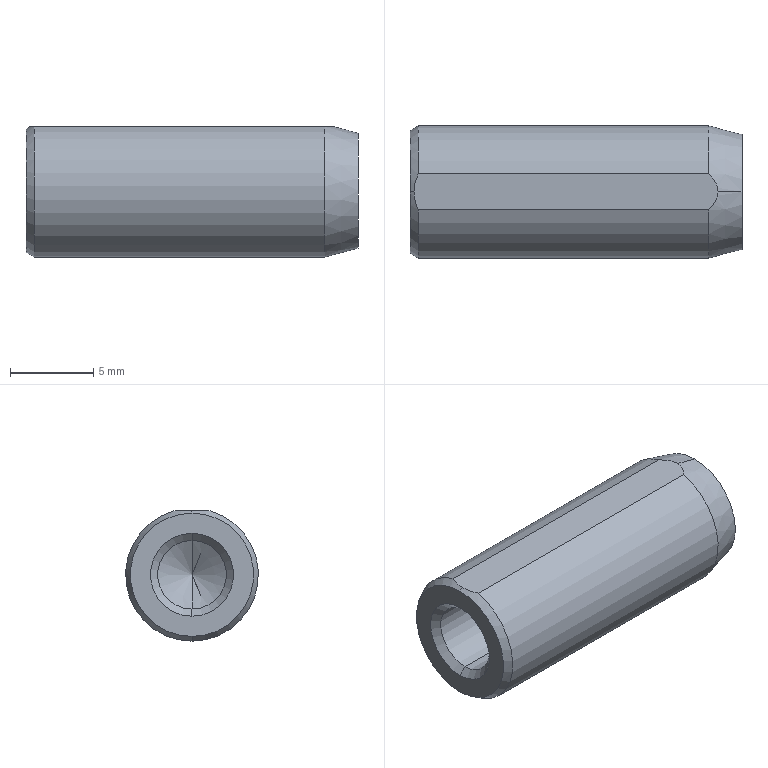Part | STEP file | MSTMS8-20-2 | 1 solid | 15 faces | box 20 x 8 x 7.85 mm | volume 856.572 mm3 | cone 8 | cylinder 4 | plane 3 | commonest cylinder face diameters 4.134 x2 8 x2
STEP:
#1=CARTESIAN_POINT('',(0.,0.,0.));
#2=DIRECTION('',(0.,0.,1.));
#3=DIRECTION('',(1.,0.,0.));
#4=AXIS2_PLACEMENT_3D('',#1,#2,#3);
#5=CARTESIAN_POINT('',(-0.7934,0.,2.067));
#6=VERTEX_POINT('',#5);
#7=CARTESIAN_POINT('',(-0.7934,0.,-2.067));
#8=VERTEX_POINT('',#7);
#9=CARTESIAN_POINT('',(-0.7934,0.,0.));
#10=DIRECTION('',(1.,0.,0.));
#11=DIRECTION('',(0.,0.,-1.));
#12=AXIS2_PLACEMENT_3D('',#9,#10,#11);
#13=CIRCLE('',#12,2.067);
#14=CARTESIAN_POINT('',(-0.7934,0.,0.));
#15=DIRECTION('',(-1.,0.,0.));
#16=DIRECTION('',(0.,0.,1.));
#17=AXIS2_PLACEMENT_3D('',#14,#15,#16);
#18=CONICAL_SURFACE('',#17,2.067,1.047);
#19=CARTESIAN_POINT('',(9.425,0.));
#20=DIRECTION('',(-1.,0.));
#21=VECTOR('',#20,1.);
#22=LINE('',#19,#21);
#23=(GEOMETRIC_REPRESENTATION_CONTEXT(2)PARAMETRIC_REPRESENTATION_CONTEXT()REPRESENTATION_CONTEXT('',''));
#24=DEFINITIONAL_REPRESENTATION('',(#22),#23);
#25=PCURVE('',#18,#24);
#26=CARTESIAN_POINT('',(0.4,0.,0.));
#27=DIRECTION('',(1.,0.,0.));
#28=DIRECTION('',(0.,0.,-1.));
#29=AXIS2_PLACEMENT_3D('',#26,#27,#28);
#30=CYLINDRICAL_SURFACE('',#29,2.067);
#31=CARTESIAN_POINT('',(0.,-1.193));
#32=DIRECTION('',(1.,0.));
#33=VECTOR('',#32,1.);
#34=LINE('',#31,#33);
#35=(GEOMETRIC_REPRESENTATION_CONTEXT(2)PARAMETRIC_REPRESENTATION_CONTEXT()REPRESENTATION_CONTEXT('',''));
#36=DEFINITIONAL_REPRESENTATION('',(#34),#35);
#37=PCURVE('',#30,#36);
#38=SURFACE_CURVE('',#13,(#25,#37),.PCURVE_S1.);
#39=EDGE_CURVE('',#6,#8,#38,.T.);
#40=ORIENTED_EDGE('',*,*,#39,.T.);
#41=CARTESIAN_POINT('',(0.4,0.,0.));
#42=VERTEX_POINT('',#41);
#43=CARTESIAN_POINT('',(-0.7934,0.,-2.067));
#44=DIRECTION('',(-0.5,0.,-0.866));
#45=VECTOR('',#44,1.);
#46=LINE('',#43,#45);
#47=CARTESIAN_POINT('',(3.142,0.));
#48=DIRECTION('',(0.,1.));
#49=VECTOR('',#48,1.);
#50=LINE('',#47,#49);
#51=(GEOMETRIC_REPRESENTATION_CONTEXT(2)PARAMETRIC_REPRESENTATION_CONTEXT()REPRESENTATION_CONTEXT('',''));
#52=DEFINITIONAL_REPRESENTATION('',(#50),#51);
#53=PCURVE('',#18,#52);
#54=CARTESIAN_POINT('',(-0.7934,0.,0.));
#55=DIRECTION('',(-1.,0.,0.));
#56=DIRECTION('',(0.,0.,1.));
#57=AXIS2_PLACEMENT_3D('',#54,#55,#56);
#58=CONICAL_SURFACE('',#57,2.067,1.047);
#59=CARTESIAN_POINT('',(3.142,0.));
#60=DIRECTION('',(0.,1.));
#61=VECTOR('',#60,1.);
#62=LINE('',#59,#61);
#63=(GEOMETRIC_REPRESENTATION_CONTEXT(2)PARAMETRIC_REPRESENTATION_CONTEXT()REPRESENTATION_CONTEXT('',''));
#64=DEFINITIONAL_REPRESENTATION('',(#62),#63);
#65=PCURVE('',#58,#64);
#66=SURFACE_CURVE('',#46,(#53,#65),.PCURVE_S1.);
#67=EDGE_CURVE('',#42,#8,#66,.T.);
#68=ORIENTED_EDGE('',*,*,#67,.F.);
#69=CARTESIAN_POINT('',(-0.7934,0.,2.067));
#70=DIRECTION('',(-0.5,0.,0.866));
#71=VECTOR('',#70,1.);
#72=LINE('',#69,#71);
#73=CARTESIAN_POINT('',(6.283,0.));
#74=DIRECTION('',(0.,1.));
#75=VECTOR('',#74,1.);
#76=LINE('',#73,#75);
#77=(GEOMETRIC_REPRESENTATION_CONTEXT(2)PARAMETRIC_REPRESENTATION_CONTEXT()REPRESENTATION_CONTEXT('',''));
#78=DEFINITIONAL_REPRESENTATION('',(#76),#77);
#79=PCURVE('',#18,#78);
#80=CARTESIAN_POINT('',(0.,0.));
#81=DIRECTION('',(0.,1.));
#82=VECTOR('',#81,1.);
#83=LINE('',#80,#82);
#84=(GEOMETRIC_REPRESENTATION_CONTEXT(2)PARAMETRIC_REPRESENTATION_CONTEXT()REPRESENTATION_CONTEXT('',''));
#85=DEFINITIONAL_REPRESENTATION('',(#83),#84);
#86=PCURVE('',#58,#85);
#87=SURFACE_CURVE('',#72,(#79,#86),.PCURVE_S1.);
#88=EDGE_CURVE('',#42,#6,#87,.T.);
#89=ORIENTED_EDGE('',*,*,#88,.T.);
#90=EDGE_LOOP('',(#40,#68,#89));
#91=FACE_BOUND('',#90,.F.);
#92=ADVANCED_FACE('',(#91),#18,.F.);
#93=CARTESIAN_POINT('',(-9.567,0.,-2.067));
#94=VERTEX_POINT('',#93);
#95=CARTESIAN_POINT('',(0.4,0.,-2.067));
#96=DIRECTION('',(1.,0.,0.));
#97=VECTOR('',#96,1.);
#98=LINE('',#95,#97);
#99=CARTESIAN_POINT('',(6.283,0.));
#100=DIRECTION('',(0.,1.));
#101=VECTOR('',#100,1.);
#102=LINE('',#99,#101);
#103=(GEOMETRIC_REPRESENTATION_CONTEXT(2)PARAMETRIC_REPRESENTATION_CONTEXT()REPRESENTATION_CONTEXT('',''));
#104=DEFINITIONAL_REPRESENTATION('',(#102),#103);
#105=PCURVE('',#30,#104);
#106=CARTESIAN_POINT('',(0.4,0.,0.));
#107=DIRECTION('',(1.,0.,0.));
#108=DIRECTION('',(0.,0.,-1.));
#109=AXIS2_PLACEMENT_3D('',#106,#107,#108);
#110=CYLINDRICAL_SURFACE('',#109,2.067);
#111=CARTESIAN_POINT('',(0.,0.));
#112=DIRECTION('',(0.,1.));
#113=VECTOR('',#112,1.);
#114=LINE('',#111,#113);
#115=(GEOMETRIC_REPRESENTATION_CONTEXT(2)PARAMETRIC_REPRESENTATION_CONTEXT()REPRESENTATION_CONTEXT('',''));
#116=DEFINITIONAL_REPRESENTATION('',(#114),#115);
#117=PCURVE('',#110,#116);
#118=SURFACE_CURVE('',#98,(#105,#117),.PCURVE_S1.);
#119=EDGE_CURVE('',#94,#8,#118,.T.);
#120=ORIENTED_EDGE('',*,*,#119,.T.);
#121=ORIENTED_EDGE('',*,*,#39,.F.);
#122=CARTESIAN_POINT('',(-9.567,0.,2.067));
#123=VERTEX_POINT('',#122);
#124=CARTESIAN_POINT('',(0.4,0.,2.067));
#125=DIRECTION('',(1.,0.,0.));
#126=VECTOR('',#125,1.);
#127=LINE('',#124,#126);
#128=CARTESIAN_POINT('',(3.142,0.));
#129=DIRECTION('',(0.,1.));
#130=VECTOR('',#129,1.);
#131=LINE('',#128,#130);
#132=(GEOMETRIC_REPRESENTATION_CONTEXT(2)PARAMETRIC_REPRESENTATION_CONTEXT()REPRESENTATION_CONTEXT('',''));
#133=DEFINITIONAL_REPRESENTATION('',(#131),#132);
#134=PCURVE('',#30,#133);
#135=CARTESIAN_POINT('',(3.142,0.));
#136=DIRECTION('',(0.,1.));
#137=VECTOR('',#136,1.);
#138=LINE('',#135,#137);
#139=(GEOMETRIC_REPRESENTATION_CONTEXT(2)PARAMETRIC_REPRESENTATION_CONTEXT()REPRESENTATION_CONTEXT('',''));
#140=DEFINITIONAL_REPRESENTATION('',(#138),#139);
#141=PCURVE('',#110,#140);
#142=SURFACE_CURVE('',#127,(#134,#141),.PCURVE_S1.);
#143=EDGE_CURVE('',#123,#6,#142,.T.);
#144=ORIENTED_EDGE('',*,*,#143,.F.);
#145=CARTESIAN_POINT('',(-9.567,0.,0.));
#146=DIRECTION('',(1.,0.,0.));
#147=DIRECTION('',(0.,0.,-1.));
#148=AXIS2_PLACEMENT_3D('',#145,#146,#147);
#149=CIRCLE('',#148,2.067);
#150=CARTESIAN_POINT('',(0.,-9.967));
#151=DIRECTION('',(1.,0.));
#152=VECTOR('',#151,1.);
#153=LINE('',#150,#152);
#154=(GEOMETRIC_REPRESENTATION_CONTEXT(2)PARAMETRIC_REPRESENTATION_CONTEXT()REPRESENTATION_CONTEXT('',''));
#155=DEFINITIONAL_REPRESENTATION('',(#153),#154);
#156=PCURVE('',#30,#155);
#157=CARTESIAN_POINT('',(-10.,0.,0.));
#158=DIRECTION('',(-1.,0.,0.));
#159=DIRECTION('',(0.,0.,1.));
#160=AXIS2_PLACEMENT_3D('',#157,#158,#159);
#161=CONICAL_SURFACE('',#160,2.5,0.7854);
#162=CARTESIAN_POINT('',(9.425,-0.433));
#163=DIRECTION('',(-1.,0.));
#164=VECTOR('',#163,1.);
#165=LINE('',#162,#164);
#166=(GEOMETRIC_REPRESENTATION_CONTEXT(2)PARAMETRIC_REPRESENTATION_CONTEXT()REPRESENTATION_CONTEXT('',''));
#167=DEFINITIONAL_REPRESENTATION('',(#165),#166);
#168=PCURVE('',#161,#167);
#169=SURFACE_CURVE('',#149,(#156,#168),.PCURVE_S1.);
#170=EDGE_CURVE('',#123,#94,#169,.T.);
#171=ORIENTED_EDGE('',*,*,#170,.T.);
#172=EDGE_LOOP('',(#120,#121,#144,#171));
#173=FACE_BOUND('',#172,.F.);
#174=ADVANCED_FACE('',(#173),#30,.F.);
#175=CARTESIAN_POINT('',(-10.,0.,2.5));
#176=VERTEX_POINT('',#175);
#177=CARTESIAN_POINT('',(-10.,0.,2.5));
#178=DIRECTION('',(-0.7071,0.,0.7071));
#179=VECTOR('',#178,1.);
#180=LINE('',#177,#179);
#181=CARTESIAN_POINT('',(6.283,0.));
#182=DIRECTION('',(0.,1.));
#183=VECTOR('',#182,1.);
#184=LINE('',#181,#183);
#185=(GEOMETRIC_REPRESENTATION_CONTEXT(2)PARAMETRIC_REPRESENTATION_CONTEXT()REPRESENTATION_CONTEXT('',''));
#186=DEFINITIONAL_REPRESENTATION('',(#184),#185);
#187=PCURVE('',#161,#186);
#188=CARTESIAN_POINT('',(-10.,0.,0.));
#189=DIRECTION('',(-1.,0.,0.));
#190=DIRECTION('',(0.,0.,1.));
#191=AXIS2_PLACEMENT_3D('',#188,#189,#190);
#192=CONICAL_SURFACE('',#191,2.5,0.7854);
#193=CARTESIAN_POINT('',(0.,0.));
#194=DIRECTION('',(0.,1.));
#195=VECTOR('',#194,1.);
#196=LINE('',#193,#195);
#197=(GEOMETRIC_REPRESENTATION_CONTEXT(2)PARAMETRIC_REPRESENTATION_CONTEXT()REPRESENTATION_CONTEXT('',''));
#198=DEFINITIONAL_REPRESENTATION('',(#196),#197);
#199=PCURVE('',#192,#198);
#200=SURFACE_CURVE('',#180,(#187,#199),.PCURVE_S1.);
#201=EDGE_CURVE('',#123,#176,#200,.T.);
#202=ORIENTED_EDGE('',*,*,#201,.T.);
#203=CARTESIAN_POINT('',(-10.,0.,-2.5));
#204=VERTEX_POINT('',#203);
#205=CARTESIAN_POINT('',(-10.,0.,0.));
#206=DIRECTION('',(1.,0.,0.));
#207=DIRECTION('',(0.,0.,-1.));
#208=AXIS2_PLACEMENT_3D('',#205,#206,#207);
#209=CIRCLE('',#208,2.5);
#210=CARTESIAN_POINT('',(9.425,0.));
#211=DIRECTION('',(-1.,0.));
#212=VECTOR('',#211,1.);
#213=LINE('',#210,#212);
#214=(GEOMETRIC_REPRESENTATION_CONTEXT(2)PARAMETRIC_REPRESENTATION_CONTEXT()REPRESENTATION_CONTEXT('',''));
#215=DEFINITIONAL_REPRESENTATION('',(#213),#214);
#216=PCURVE('',#161,#215);
#217=CARTESIAN_POINT('',(-10.,0.,0.));
#218=DIRECTION('',(1.,0.,0.));
#219=DIRECTION('',(0.,0.,-1.));
#220=AXIS2_PLACEMENT_3D('',#217,#218,#219);
#221=PLANE('',#220);
#222=CARTESIAN_POINT('',(0.,0.));
#223=DIRECTION('',(1.,0.));
#224=AXIS2_PLACEMENT_2D('',#222,#223);
#225=CIRCLE('',#224,2.5);
#226=(GEOMETRIC_REPRESENTATION_CONTEXT(2)PARAMETRIC_REPRESENTATION_CONTEXT()REPRESENTATION_CONTEXT('',''));
#227=DEFINITIONAL_REPRESENTATION('',(#225),#226);
#228=PCURVE('',#221,#227);
#229=SURFACE_CURVE('',#209,(#216,#228),.PCURVE_S1.);
#230=EDGE_CURVE('',#176,#204,#229,.T.);
#231=ORIENTED_EDGE('',*,*,#230,.T.);
#232=CARTESIAN_POINT('',(-10.,0.,-2.5));
#233=DIRECTION('',(-0.7071,0.,-0.7071));
#234=VECTOR('',#233,1.);
#235=LINE('',#232,#234);
#236=CARTESIAN_POINT('',(3.142,0.));
#237=DIRECTION('',(0.,1.));
#238=VECTOR('',#237,1.);
#239=LINE('',#236,#238);
#240=(GEOMETRIC_REPRESENTATION_CONTEXT(2)PARAMETRIC_REPRESENTATION_CONTEXT()REPRESENTATION_CONTEXT('',''));
#241=DEFINITIONAL_REPRESENTATION('',(#239),#240);
#242=PCURVE('',#161,#241);
#243=CARTESIAN_POINT('',(3.142,0.));
#244=DIRECTION('',(0.,1.));
#245=VECTOR('',#244,1.);
#246=LINE('',#243,#245);
#247=(GEOMETRIC_REPRESENTATION_CONTEXT(2)PARAMETRIC_REPRESENTATION_CONTEXT()REPRESENTATION_CONTEXT('',''));
#248=DEFINITIONAL_REPRESENTATION('',(#246),#247);
#249=PCURVE('',#192,#248);
#250=SURFACE_CURVE('',#235,(#242,#249),.PCURVE_S1.);
#251=EDGE_CURVE('',#94,#204,#250,.T.);
#252=ORIENTED_EDGE('',*,*,#251,.F.);
#253=ORIENTED_EDGE('',*,*,#170,.F.);
#254=EDGE_LOOP('',(#202,#231,#252,#253));
#255=FACE_BOUND('',#254,.F.);
#256=ADVANCED_FACE('',(#255),#161,.F.);
#257=CARTESIAN_POINT('',(10.,0.,-3.464));
#258=VERTEX_POINT('',#257);
#259=CARTESIAN_POINT('',(10.,0.,3.464));
#260=VERTEX_POINT('',#259);
#261=CARTESIAN_POINT('',(10.,0.,0.));
#262=DIRECTION('',(1.,0.,0.));
#263=DIRECTION('',(0.,0.,-1.));
#264=AXIS2_PLACEMENT_3D('',#261,#262,#263);
#265=CIRCLE('',#264,3.464);
#266=CARTESIAN_POINT('',(8.,0.,0.));
#267=DIRECTION('',(-1.,0.,0.));
#268=DIRECTION('',(0.,0.,1.));
#269=AXIS2_PLACEMENT_3D('',#266,#267,#268);
#270=CONICAL_SURFACE('',#269,4.,0.2618);
#271=CARTESIAN_POINT('',(3.142,-2.));
#272=DIRECTION('',(-1.,0.));
#273=VECTOR('',#272,1.);
#274=LINE('',#271,#273);
#275=(GEOMETRIC_REPRESENTATION_CONTEXT(2)PARAMETRIC_REPRESENTATION_CONTEXT()REPRESENTATION_CONTEXT('',''));
#276=DEFINITIONAL_REPRESENTATION('',(#274),#275);
#277=PCURVE('',#270,#276);
#278=CARTESIAN_POINT('',(10.,3.464,0.));
#279=DIRECTION('',(-1.,0.,0.));
#280=DIRECTION('',(0.,0.,1.));
#281=AXIS2_PLACEMENT_3D('',#278,#279,#280);
#282=PLANE('',#281);
#283=CARTESIAN_POINT('',(-3.464,-3.464));
#284=CARTESIAN_POINT('',(-3.464,2.536));
#285=CARTESIAN_POINT('',(1.732,-0.4641));
#286=CARTESIAN_POINT('',(6.928,-3.464));
#287=CARTESIAN_POINT('',(1.732,-6.464));
#288=CARTESIAN_POINT('',(-3.464,-9.464));
#289=CARTESIAN_POINT('',(-3.464,-3.464));
#290=(BOUNDED_CURVE()B_SPLINE_CURVE(2,(#283,#284,#285,#286,#287,#288,#289),.UNSPECIFIED.,.T.,.F.)B_SPLINE_CURVE_WITH_KNOTS((1,2,2,2,2,1),(-2.094,0.,2.094,4.189,6.283,8.378),.UNSPECIFIED.)CURVE()GEOMETRIC_REPRESENTATION_ITEM()RATIONAL_B_SPLINE_CURVE((1.,0.5,1.,0.5,1.,0.5,1.))REPRESENTATION_ITEM(''));
#291=(GEOMETRIC_REPRESENTATION_CONTEXT(2)PARAMETRIC_REPRESENTATION_CONTEXT()REPRESENTATION_CONTEXT('',''));
#292=DEFINITIONAL_REPRESENTATION('',(#290),#291);
#293=PCURVE('',#282,#292);
#294=SURFACE_CURVE('',#265,(#277,#293),.PCURVE_S1.);
#295=EDGE_CURVE('',#258,#260,#294,.T.);
#296=ORIENTED_EDGE('',*,*,#295,.F.);
#297=CARTESIAN_POINT('',(8.,0.,-4.));
#298=VERTEX_POINT('',#297);
#299=CARTESIAN_POINT('',(8.,0.,-4.));
#300=DIRECTION('',(-0.9659,0.,-0.2588));
#301=VECTOR('',#300,1.);
#302=LINE('',#299,#301);
#303=CARTESIAN_POINT('',(3.142,0.));
#304=DIRECTION('',(0.,1.));
#305=VECTOR('',#304,1.);
#306=LINE('',#303,#305);
#307=(GEOMETRIC_REPRESENTATION_CONTEXT(2)PARAMETRIC_REPRESENTATION_CONTEXT()REPRESENTATION_CONTEXT('',''));
#308=DEFINITIONAL_REPRESENTATION('',(#306),#307);
#309=PCURVE('',#270,#308);
#310=CARTESIAN_POINT('',(8.,0.,0.));
#311=DIRECTION('',(-1.,0.,0.));
#312=DIRECTION('',(0.,0.,1.));
#313=AXIS2_PLACEMENT_3D('',#310,#311,#312);
#314=CONICAL_SURFACE('',#313,4.,0.2618);
#315=CARTESIAN_POINT('',(3.142,0.));
#316=DIRECTION('',(0.,1.));
#317=VECTOR('',#316,1.);
#318=LINE('',#315,#317);
#319=(GEOMETRIC_REPRESENTATION_CONTEXT(2)PARAMETRIC_REPRESENTATION_CONTEXT()REPRESENTATION_CONTEXT('',''));
#320=DEFINITIONAL_REPRESENTATION('',(#318),#319);
#321=PCURVE('',#314,#320);
#322=SURFACE_CURVE('',#302,(#309,#321),.PCURVE_S1.);
#323=EDGE_CURVE('',#258,#298,#322,.T.);
#324=ORIENTED_EDGE('',*,*,#323,.T.);
#325=CARTESIAN_POINT('',(8.,1.085,3.85));
#326=VERTEX_POINT('',#325);
#327=CARTESIAN_POINT('',(8.,0.,0.));
#328=DIRECTION('',(1.,0.,0.));
#329=DIRECTION('',(0.,0.,-1.));
#330=AXIS2_PLACEMENT_3D('',#327,#328,#329);
#331=CIRCLE('',#330,4.);
#332=CARTESIAN_POINT('',(3.142,0.));
#333=DIRECTION('',(-1.,0.));
#334=VECTOR('',#333,1.);
#335=LINE('',#332,#334);
#336=(GEOMETRIC_REPRESENTATION_CONTEXT(2)PARAMETRIC_REPRESENTATION_CONTEXT()REPRESENTATION_CONTEXT('',''));
#337=DEFINITIONAL_REPRESENTATION('',(#335),#336);
#338=PCURVE('',#270,#337);
#339=CARTESIAN_POINT('',(10.,0.,0.));
#340=DIRECTION('',(1.,0.,0.));
#341=DIRECTION('',(0.,0.,-1.));
#342=AXIS2_PLACEMENT_3D('',#339,#340,#341);
#343=CYLINDRICAL_SURFACE('',#342,4.);
#344=CARTESIAN_POINT('',(0.,-2.));
#345=DIRECTION('',(1.,0.));
#346=VECTOR('',#345,1.);
#347=LINE('',#344,#346);
#348=(GEOMETRIC_REPRESENTATION_CONTEXT(2)PARAMETRIC_REPRESENTATION_CONTEXT()REPRESENTATION_CONTEXT('',''));
#349=DEFINITIONAL_REPRESENTATION('',(#347),#348);
#350=PCURVE('',#343,#349);
#351=SURFACE_CURVE('',#331,(#338,#350),.PCURVE_S1.);
#352=EDGE_CURVE('',#298,#326,#351,.T.);
#353=ORIENTED_EDGE('',*,*,#352,.T.);
#354=CARTESIAN_POINT('',(8.56,0.,3.85));
#355=VERTEX_POINT('',#354);
#356=CARTESIAN_POINT('',(8.56,0.,3.85));
#357=CARTESIAN_POINT('',(8.56,0.1037,3.85));
#358=CARTESIAN_POINT('',(8.543,0.2093,3.85));
#359=CARTESIAN_POINT('',(8.484,0.4095,3.85));
#360=CARTESIAN_POINT('',(8.44,0.5063,3.85));
#361=CARTESIAN_POINT('',(8.284,0.7783,3.85));
#362=CARTESIAN_POINT('',(8.148,0.9387,3.85));
#363=CARTESIAN_POINT('',(8.,1.085,3.85));
#364=B_SPLINE_CURVE_WITH_KNOTS('',3,(#356,#357,#358,#359,#360,#361,#362,#363),.UNSPECIFIED.,.F.,.F.,(4,2,2,4),(0.01037,0.01068,0.01099,0.01162),.UNSPECIFIED.);
#365=CARTESIAN_POINT('',(0.,-0.5598));
#366=CARTESIAN_POINT('',(0.004899,-0.5598));
#367=CARTESIAN_POINT('',(0.01473,-0.5587));
#368=CARTESIAN_POINT('',(0.02949,-0.554));
#369=CARTESIAN_POINT('',(0.04421,-0.5461));
#370=CARTESIAN_POINT('',(0.05879,-0.5354));
#371=CARTESIAN_POINT('',(0.07317,-0.5218));
#372=CARTESIAN_POINT('',(0.08725,-0.5054));
#373=CARTESIAN_POINT('',(0.1011,-0.4865));
#374=CARTESIAN_POINT('',(0.1148,-0.4651));
#375=CARTESIAN_POINT('',(0.1281,-0.4415));
#376=CARTESIAN_POINT('',(0.1412,-0.4159));
#377=CARTESIAN_POINT('',(0.1539,-0.3884));
#378=CARTESIAN_POINT('',(0.1663,-0.3593));
#379=CARTESIAN_POINT('',(0.1784,-0.3287));
#380=CARTESIAN_POINT('',(0.1901,-0.2966));
#381=CARTESIAN_POINT('',(0.2016,-0.2633));
#382=CARTESIAN_POINT('',(0.2129,-0.2287));
#383=CARTESIAN_POINT('',(0.2238,-0.1929));
#384=CARTESIAN_POINT('',(0.2345,-0.1561));
#385=CARTESIAN_POINT('',(0.2449,-0.1183));
#386=CARTESIAN_POINT('',(0.2551,-0.07967));
#387=CARTESIAN_POINT('',(0.265,-0.04024));
#388=CARTESIAN_POINT('',(0.2715,-0.01348));
#389=CARTESIAN_POINT('',(0.2747,0.));
#390=B_SPLINE_CURVE_WITH_KNOTS('',3,(#365,#366,#367,#368,#369,#370,#371,#372,#373,#374,#375,#376,#377,#378,#379,#380,#381,#382,#383,#384,#385,#386,#387,#388,#389),.UNSPECIFIED.,.F.,.F.,(4,1,1,1,1,1,1,1,1,1,1,1,1,1,1,1,1,1,1,1,1,1,4),(0.01037,0.01043,0.01048,0.01054,0.0106,0.01065,0.01071,0.01077,0.01082,0.01088,0.01094,0.01099,0.01105,0.01111,0.01116,0.01122,0.01128,0.01133,0.01139,0.01145,0.0115,0.01156,0.01162),.QUASI_UNIFORM_KNOTS.);
#391=(GEOMETRIC_REPRESENTATION_CONTEXT(2)PARAMETRIC_REPRESENTATION_CONTEXT()REPRESENTATION_CONTEXT('',''));
#392=DEFINITIONAL_REPRESENTATION('',(#390),#391);
#393=PCURVE('',#270,#392);
#394=CARTESIAN_POINT('',(10.,-4.,3.85));
#395=DIRECTION('',(0.,0.,1.));
#396=DIRECTION('',(1.,0.,0.));
#397=AXIS2_PLACEMENT_3D('',#394,#395,#396);
#398=PLANE('',#397);
#399=CARTESIAN_POINT('',(-1.44,4.));
#400=CARTESIAN_POINT('',(-1.44,4.104));
#401=CARTESIAN_POINT('',(-1.457,4.209));
#402=CARTESIAN_POINT('',(-1.516,4.41));
#403=CARTESIAN_POINT('',(-1.56,4.506));
#404=CARTESIAN_POINT('',(-1.716,4.778));
#405=CARTESIAN_POINT('',(-1.852,4.939));
#406=CARTESIAN_POINT('',(-2.,5.085));
#407=B_SPLINE_CURVE_WITH_KNOTS('',3,(#399,#400,#401,#402,#403,#404,#405,#406),.UNSPECIFIED.,.F.,.F.,(4,2,2,4),(0.01037,0.01068,0.01099,0.01162),.UNSPECIFIED.);
#408=(GEOMETRIC_REPRESENTATION_CONTEXT(2)PARAMETRIC_REPRESENTATION_CONTEXT()REPRESENTATION_CONTEXT('',''));
#409=DEFINITIONAL_REPRESENTATION('',(#407),#408);
#410=PCURVE('',#398,#409);
#411=SURFACE_CURVE('',#364,(#393,#410),.PCURVE_S1.);
#412=EDGE_CURVE('',#355,#326,#411,.T.);
#413=ORIENTED_EDGE('',*,*,#412,.F.);
#414=CARTESIAN_POINT('',(8.,0.,4.));
#415=DIRECTION('',(-0.9659,0.,0.2588));
#416=VECTOR('',#415,1.);
#417=LINE('',#414,#416);
#418=CARTESIAN_POINT('',(0.,0.));
#419=DIRECTION('',(0.,1.));
#420=VECTOR('',#419,1.);
#421=LINE('',#418,#420);
#422=(GEOMETRIC_REPRESENTATION_CONTEXT(2)PARAMETRIC_REPRESENTATION_CONTEXT()REPRESENTATION_CONTEXT('',''));
#423=DEFINITIONAL_REPRESENTATION('',(#421),#422);
#424=PCURVE('',#270,#423);
#425=CARTESIAN_POINT('',(6.283,0.));
#426=DIRECTION('',(0.,1.));
#427=VECTOR('',#426,1.);
#428=LINE('',#425,#427);
#429=(GEOMETRIC_REPRESENTATION_CONTEXT(2)PARAMETRIC_REPRESENTATION_CONTEXT()REPRESENTATION_CONTEXT('',''));
#430=DEFINITIONAL_REPRESENTATION('',(#428),#429);
#431=PCURVE('',#314,#430);
#432=SURFACE_CURVE('',#417,(#424,#431),.PCURVE_S1.);
#433=EDGE_CURVE('',#260,#355,#432,.T.);
#434=ORIENTED_EDGE('',*,*,#433,.F.);
#435=EDGE_LOOP('',(#296,#324,#353,#413,#434));
#436=FACE_BOUND('',#435,.T.);
#437=ADVANCED_FACE('',(#436),#270,.T.);
#438=CARTESIAN_POINT('',(-9.5,-1.085,3.85));
#439=VERTEX_POINT('',#438);
#440=CARTESIAN_POINT('',(-9.5,0.,-4.));
#441=VERTEX_POINT('',#440);
#442=CARTESIAN_POINT('',(-9.5,0.,0.));
#443=DIRECTION('',(1.,0.,0.));
#444=DIRECTION('',(0.,0.,-1.));
#445=AXIS2_PLACEMENT_3D('',#442,#443,#444);
#446=CIRCLE('',#445,4.);
#447=CARTESIAN_POINT('',(10.,0.,0.));
#448=DIRECTION('',(1.,0.,0.));
#449=DIRECTION('',(0.,0.,-1.));
#450=AXIS2_PLACEMENT_3D('',#447,#448,#449);
#451=CYLINDRICAL_SURFACE('',#450,4.);
#452=CARTESIAN_POINT('',(0.,-19.5));
#453=DIRECTION('',(1.,0.));
#454=VECTOR('',#453,1.);
#455=LINE('',#452,#454);
#456=(GEOMETRIC_REPRESENTATION_CONTEXT(2)PARAMETRIC_REPRESENTATION_CONTEXT()REPRESENTATION_CONTEXT('',''));
#457=DEFINITIONAL_REPRESENTATION('',(#455),#456);
#458=PCURVE('',#451,#457);
#459=CARTESIAN_POINT('',(-10.,0.,0.));
#460=DIRECTION('',(1.,0.,0.));
#461=DIRECTION('',(0.,0.,-1.));
#462=AXIS2_PLACEMENT_3D('',#459,#460,#461);
#463=CONICAL_SURFACE('',#462,3.711,0.5236);
#464=CARTESIAN_POINT('',(0.,0.5));
#465=DIRECTION('',(1.,0.));
#466=VECTOR('',#465,1.);
#467=LINE('',#464,#466);
#468=(GEOMETRIC_REPRESENTATION_CONTEXT(2)PARAMETRIC_REPRESENTATION_CONTEXT()REPRESENTATION_CONTEXT('',''));
#469=DEFINITIONAL_REPRESENTATION('',(#467),#468);
#470=PCURVE('',#463,#469);
#471=SURFACE_CURVE('',#446,(#458,#470),.PCURVE_S1.);
#472=EDGE_CURVE('',#439,#441,#471,.T.);
#473=ORIENTED_EDGE('',*,*,#472,.T.);
#474=CARTESIAN_POINT('',(10.,0.,-4.));
#475=DIRECTION('',(1.,0.,0.));
#476=VECTOR('',#475,1.);
#477=LINE('',#474,#476);
#478=CARTESIAN_POINT('',(6.283,0.));
#479=DIRECTION('',(0.,1.));
#480=VECTOR('',#479,1.);
#481=LINE('',#478,#480);
#482=(GEOMETRIC_REPRESENTATION_CONTEXT(2)PARAMETRIC_REPRESENTATION_CONTEXT()REPRESENTATION_CONTEXT('',''));
#483=DEFINITIONAL_REPRESENTATION('',(#481),#482);
#484=PCURVE('',#451,#483);
#485=CARTESIAN_POINT('',(0.,0.));
#486=DIRECTION('',(0.,1.));
#487=VECTOR('',#486,1.);
#488=LINE('',#485,#487);
#489=(GEOMETRIC_REPRESENTATION_CONTEXT(2)PARAMETRIC_REPRESENTATION_CONTEXT()REPRESENTATION_CONTEXT('',''));
#490=DEFINITIONAL_REPRESENTATION('',(#488),#489);
#491=PCURVE('',#343,#490);
#492=SURFACE_CURVE('',#477,(#484,#491),.PCURVE_S1.);
#493=EDGE_CURVE('',#441,#298,#492,.T.);
#494=ORIENTED_EDGE('',*,*,#493,.T.);
#495=CARTESIAN_POINT('',(8.,-1.085,3.85));
#496=VERTEX_POINT('',#495);
#497=CARTESIAN_POINT('',(8.,0.,0.));
#498=DIRECTION('',(1.,0.,0.));
#499=DIRECTION('',(0.,0.,-1.));
#500=AXIS2_PLACEMENT_3D('',#497,#498,#499);
#501=CIRCLE('',#500,4.);
#502=CARTESIAN_POINT('',(0.,-2.));
#503=DIRECTION('',(1.,0.));
#504=VECTOR('',#503,1.);
#505=LINE('',#502,#504);
#506=(GEOMETRIC_REPRESENTATION_CONTEXT(2)PARAMETRIC_REPRESENTATION_CONTEXT()REPRESENTATION_CONTEXT('',''));
#507=DEFINITIONAL_REPRESENTATION('',(#505),#506);
#508=PCURVE('',#451,#507);
#509=CARTESIAN_POINT('',(9.425,0.));
#510=DIRECTION('',(-1.,0.));
#511=VECTOR('',#510,1.);
#512=LINE('',#509,#511);
#513=(GEOMETRIC_REPRESENTATION_CONTEXT(2)PARAMETRIC_REPRESENTATION_CONTEXT()REPRESENTATION_CONTEXT('',''));
#514=DEFINITIONAL_REPRESENTATION('',(#512),#513);
#515=PCURVE('',#314,#514);
#516=SURFACE_CURVE('',#501,(#508,#515),.PCURVE_S1.);
#517=EDGE_CURVE('',#496,#298,#516,.T.);
#518=ORIENTED_EDGE('',*,*,#517,.F.);
#519=CARTESIAN_POINT('',(10.,-1.085,3.85));
#520=DIRECTION('',(1.,0.,0.));
#521=VECTOR('',#520,1.);
#522=LINE('',#519,#521);
#523=CARTESIAN_POINT('',(3.416,0.));
#524=DIRECTION('',(0.,1.));
#525=VECTOR('',#524,1.);
#526=LINE('',#523,#525);
#527=(GEOMETRIC_REPRESENTATION_CONTEXT(2)PARAMETRIC_REPRESENTATION_CONTEXT()REPRESENTATION_CONTEXT('',''));
#528=DEFINITIONAL_REPRESENTATION('',(#526),#527);
#529=PCURVE('',#451,#528);
#530=CARTESIAN_POINT('',(0.,2.915));
#531=DIRECTION('',(1.,0.));
#532=VECTOR('',#531,1.);
#533=LINE('',#530,#532);
#534=(GEOMETRIC_REPRESENTATION_CONTEXT(2)PARAMETRIC_REPRESENTATION_CONTEXT()REPRESENTATION_CONTEXT('',''));
#535=DEFINITIONAL_REPRESENTATION('',(#533),#534);
#536=PCURVE('',#398,#535);
#537=SURFACE_CURVE('',#522,(#529,#536),.PCURVE_S1.);
#538=EDGE_CURVE('',#439,#496,#537,.T.);
#539=ORIENTED_EDGE('',*,*,#538,.F.);
#540=EDGE_LOOP('',(#473,#494,#518,#539));
#541=FACE_BOUND('',#540,.T.);
#542=ADVANCED_FACE('',(#541),#451,.T.);
#543=CARTESIAN_POINT('',(-10.,0.,-3.711));
#544=VERTEX_POINT('',#543);
#545=CARTESIAN_POINT('',(-10.,0.,3.711));
#546=VERTEX_POINT('',#545);
#547=CARTESIAN_POINT('',(-10.,0.,0.));
#548=DIRECTION('',(1.,0.,0.));
#549=DIRECTION('',(0.,0.,-1.));
#550=AXIS2_PLACEMENT_3D('',#547,#548,#549);
#551=CIRCLE('',#550,3.711);
#552=CARTESIAN_POINT('',(-10.,0.,0.));
#553=DIRECTION('',(1.,0.,0.));
#554=DIRECTION('',(0.,0.,-1.));
#555=AXIS2_PLACEMENT_3D('',#552,#553,#554);
#556=CONICAL_SURFACE('',#555,3.711,0.5236);
#557=CARTESIAN_POINT('',(0.,0.));
#558=DIRECTION('',(1.,0.));
#559=VECTOR('',#558,1.);
#560=LINE('',#557,#559);
#561=(GEOMETRIC_REPRESENTATION_CONTEXT(2)PARAMETRIC_REPRESENTATION_CONTEXT()REPRESENTATION_CONTEXT('',''));
#562=DEFINITIONAL_REPRESENTATION('',(#560),#561);
#563=PCURVE('',#556,#562);
#564=CARTESIAN_POINT('',(0.,0.));
#565=DIRECTION('',(1.,0.));
#566=AXIS2_PLACEMENT_2D('',#564,#565);
#567=CIRCLE('',#566,3.711);
#568=(GEOMETRIC_REPRESENTATION_CONTEXT(2)PARAMETRIC_REPRESENTATION_CONTEXT()REPRESENTATION_CONTEXT('',''));
#569=DEFINITIONAL_REPRESENTATION('',(#567),#568);
#570=PCURVE('',#221,#569);
#571=SURFACE_CURVE('',#551,(#563,#570),.PCURVE_S1.);
#572=EDGE_CURVE('',#544,#546,#571,.T.);
#573=ORIENTED_EDGE('',*,*,#572,.T.);
#574=CARTESIAN_POINT('',(-9.76,0.,3.85));
#575=VERTEX_POINT('',#574);
#576=CARTESIAN_POINT('',(-10.,0.,3.711));
#577=DIRECTION('',(0.866,0.,0.5));
#578=VECTOR('',#577,1.);
#579=LINE('',#576,#578);
#580=CARTESIAN_POINT('',(3.142,0.));
#581=DIRECTION('',(0.,1.));
#582=VECTOR('',#581,1.);
#583=LINE('',#580,#582);
#584=(GEOMETRIC_REPRESENTATION_CONTEXT(2)PARAMETRIC_REPRESENTATION_CONTEXT()REPRESENTATION_CONTEXT('',''));
#585=DEFINITIONAL_REPRESENTATION('',(#583),#584);
#586=PCURVE('',#556,#585);
#587=CARTESIAN_POINT('',(3.142,0.));
#588=DIRECTION('',(0.,1.));
#589=VECTOR('',#588,1.);
#590=LINE('',#587,#589);
#591=(GEOMETRIC_REPRESENTATION_CONTEXT(2)PARAMETRIC_REPRESENTATION_CONTEXT()REPRESENTATION_CONTEXT('',''));
#592=DEFINITIONAL_REPRESENTATION('',(#590),#591);
#593=PCURVE('',#463,#592);
#594=SURFACE_CURVE('',#579,(#586,#593),.PCURVE_S1.);
#595=EDGE_CURVE('',#546,#575,#594,.T.);
#596=ORIENTED_EDGE('',*,*,#595,.T.);
#597=CARTESIAN_POINT('',(-9.5,1.085,3.85));
#598=VERTEX_POINT('',#597);
#599=CARTESIAN_POINT('',(-9.5,1.085,3.85));
#600=CARTESIAN_POINT('',(-9.58,0.915,3.85));
#601=CARTESIAN_POINT('',(-9.645,0.7396,3.85));
#602=CARTESIAN_POINT('',(-9.736,0.3748,3.85));
#603=CARTESIAN_POINT('',(-9.76,0.1861,3.85));
#604=CARTESIAN_POINT('',(-9.76,0.,3.85));
#605=B_SPLINE_CURVE_WITH_KNOTS('',3,(#599,#600,#601,#602,#603,#604),.UNSPECIFIED.,.F.,.F.,(4,2,4),(0.0105,0.01106,0.01162),.UNSPECIFIED.);
#606=CARTESIAN_POINT('',(2.867,0.5));
#607=CARTESIAN_POINT('',(2.871,0.4927));
#608=CARTESIAN_POINT('',(2.878,0.4784));
#609=CARTESIAN_POINT('',(2.889,0.4578));
#610=CARTESIAN_POINT('',(2.901,0.4379));
#611=CARTESIAN_POINT('',(2.913,0.4188));
#612=CARTESIAN_POINT('',(2.924,0.4005));
#613=CARTESIAN_POINT('',(2.936,0.3831));
#614=CARTESIAN_POINT('',(2.948,0.3665));
#615=CARTESIAN_POINT('',(2.96,0.3509));
#616=CARTESIAN_POINT('',(2.973,0.3361));
#617=CARTESIAN_POINT('',(2.985,0.3223));
#618=CARTESIAN_POINT('',(2.998,0.3095));
#619=CARTESIAN_POINT('',(3.011,0.2977));
#620=CARTESIAN_POINT('',(3.023,0.2869));
#621=CARTESIAN_POINT('',(3.036,0.2772));
#622=CARTESIAN_POINT('',(3.049,0.2686));
#623=CARTESIAN_POINT('',(3.062,0.2611));
#624=CARTESIAN_POINT('',(3.076,0.2547));
#625=CARTESIAN_POINT('',(3.089,0.2494));
#626=CARTESIAN_POINT('',(3.102,0.2453));
#627=CARTESIAN_POINT('',(3.115,0.2424));
#628=CARTESIAN_POINT('',(3.128,0.2406));
#629=CARTESIAN_POINT('',(3.137,0.2402));
#630=CARTESIAN_POINT('',(3.142,0.2402));
#631=B_SPLINE_CURVE_WITH_KNOTS('',3,(#606,#607,#608,#609,#610,#611,#612,#613,#614,#615,#616,#617,#618,#619,#620,#621,#622,#623,#624,#625,#626,#627,#628,#629,#630),.UNSPECIFIED.,.F.,.F.,(4,1,1,1,1,1,1,1,1,1,1,1,1,1,1,1,1,1,1,1,1,1,4),(0.0105,0.01055,0.0106,0.01065,0.0107,0.01076,0.01081,0.01086,0.01091,0.01096,0.01101,0.01106,0.01111,0.01116,0.01121,0.01127,0.01132,0.01137,0.01142,0.01147,0.01152,0.01157,0.01162),.QUASI_UNIFORM_KNOTS.);
#632=(GEOMETRIC_REPRESENTATION_CONTEXT(2)PARAMETRIC_REPRESENTATION_CONTEXT()REPRESENTATION_CONTEXT('',''));
#633=DEFINITIONAL_REPRESENTATION('',(#631),#632);
#634=PCURVE('',#556,#633);
#635=CARTESIAN_POINT('',(-19.5,5.085));
#636=CARTESIAN_POINT('',(-19.58,4.915));
#637=CARTESIAN_POINT('',(-19.645,4.74));
#638=CARTESIAN_POINT('',(-19.736,4.375));
#639=CARTESIAN_POINT('',(-19.76,4.186));
#640=CARTESIAN_POINT('',(-19.76,4.));
#641=B_SPLINE_CURVE_WITH_KNOTS('',3,(#635,#636,#637,#638,#639,#640),.UNSPECIFIED.,.F.,.F.,(4,2,4),(0.0105,0.01106,0.01162),.UNSPECIFIED.);
#642=(GEOMETRIC_REPRESENTATION_CONTEXT(2)PARAMETRIC_REPRESENTATION_CONTEXT()REPRESENTATION_CONTEXT('',''));
#643=DEFINITIONAL_REPRESENTATION('',(#641),#642);
#644=PCURVE('',#398,#643);
#645=SURFACE_CURVE('',#605,(#634,#644),.PCURVE_S1.);
#646=EDGE_CURVE('',#598,#575,#645,.T.);
#647=ORIENTED_EDGE('',*,*,#646,.F.);
#648=CARTESIAN_POINT('',(-9.5,0.,0.));
#649=DIRECTION('',(1.,0.,0.));
#650=DIRECTION('',(0.,0.,-1.));
#651=AXIS2_PLACEMENT_3D('',#648,#649,#650);
#652=CIRCLE('',#651,4.);
#653=CARTESIAN_POINT('',(0.,0.5));
#654=DIRECTION('',(1.,0.));
#655=VECTOR('',#654,1.);
#656=LINE('',#653,#655);
#657=(GEOMETRIC_REPRESENTATION_CONTEXT(2)PARAMETRIC_REPRESENTATION_CONTEXT()REPRESENTATION_CONTEXT('',''));
#658=DEFINITIONAL_REPRESENTATION('',(#656),#657);
#659=PCURVE('',#556,#658);
#660=CARTESIAN_POINT('',(0.,-19.5));
#661=DIRECTION('',(1.,0.));
#662=VECTOR('',#661,1.);
#663=LINE('',#660,#662);
#664=(GEOMETRIC_REPRESENTATION_CONTEXT(2)PARAMETRIC_REPRESENTATION_CONTEXT()REPRESENTATION_CONTEXT('',''));
#665=DEFINITIONAL_REPRESENTATION('',(#663),#664);
#666=PCURVE('',#343,#665);
#667=SURFACE_CURVE('',#652,(#659,#666),.PCURVE_S1.);
#668=EDGE_CURVE('',#441,#598,#667,.T.);
#669=ORIENTED_EDGE('',*,*,#668,.F.);
#670=CARTESIAN_POINT('',(-10.,0.,-3.711));
#671=DIRECTION('',(0.866,0.,-0.5));
#672=VECTOR('',#671,1.);
#673=LINE('',#670,#672);
#674=CARTESIAN_POINT('',(0.,0.));
#675=DIRECTION('',(0.,1.));
#676=VECTOR('',#675,1.);
#677=LINE('',#674,#676);
#678=(GEOMETRIC_REPRESENTATION_CONTEXT(2)PARAMETRIC_REPRESENTATION_CONTEXT()REPRESENTATION_CONTEXT('',''));
#679=DEFINITIONAL_REPRESENTATION('',(#677),#678);
#680=PCURVE('',#556,#679);
#681=CARTESIAN_POINT('',(6.283,0.));
#682=DIRECTION('',(0.,1.));
#683=VECTOR('',#682,1.);
#684=LINE('',#681,#683);
#685=(GEOMETRIC_REPRESENTATION_CONTEXT(2)PARAMETRIC_REPRESENTATION_CONTEXT()REPRESENTATION_CONTEXT('',''));
#686=DEFINITIONAL_REPRESENTATION('',(#684),#685);
#687=PCURVE('',#463,#686);
#688=SURFACE_CURVE('',#673,(#680,#687),.PCURVE_S1.);
#689=EDGE_CURVE('',#544,#441,#688,.T.);
#690=ORIENTED_EDGE('',*,*,#689,.F.);
#691=EDGE_LOOP('',(#573,#596,#647,#669,#690));
#692=FACE_BOUND('',#691,.T.);
#693=ADVANCED_FACE('',(#692),#556,.T.);
#694=ORIENTED_EDGE('',*,*,#595,.F.);
#695=CARTESIAN_POINT('',(-10.,0.,0.));
#696=DIRECTION('',(1.,0.,0.));
#697=DIRECTION('',(0.,0.,-1.));
#698=AXIS2_PLACEMENT_3D('',#695,#696,#697);
#699=CIRCLE('',#698,3.711);
#700=CARTESIAN_POINT('',(0.,0.));
#701=DIRECTION('',(1.,0.));
#702=VECTOR('',#701,1.);
#703=LINE('',#700,#702);
#704=(GEOMETRIC_REPRESENTATION_CONTEXT(2)PARAMETRIC_REPRESENTATION_CONTEXT()REPRESENTATION_CONTEXT('',''));
#705=DEFINITIONAL_REPRESENTATION('',(#703),#704);
#706=PCURVE('',#463,#705);
#707=CARTESIAN_POINT('',(0.,0.));
#708=DIRECTION('',(1.,0.));
#709=AXIS2_PLACEMENT_2D('',#707,#708);
#710=CIRCLE('',#709,3.711);
#711=(GEOMETRIC_REPRESENTATION_CONTEXT(2)PARAMETRIC_REPRESENTATION_CONTEXT()REPRESENTATION_CONTEXT('',''));
#712=DEFINITIONAL_REPRESENTATION('',(#710),#711);
#713=PCURVE('',#221,#712);
#714=SURFACE_CURVE('',#699,(#706,#713),.PCURVE_S1.);
#715=EDGE_CURVE('',#546,#544,#714,.T.);
#716=ORIENTED_EDGE('',*,*,#715,.T.);
#717=ORIENTED_EDGE('',*,*,#689,.T.);
#718=ORIENTED_EDGE('',*,*,#472,.F.);
#719=CARTESIAN_POINT('',(-9.76,0.,3.85));
#720=CARTESIAN_POINT('',(-9.76,-0.1864,3.85));
#721=CARTESIAN_POINT('',(-9.736,-0.3746,3.85));
#722=CARTESIAN_POINT('',(-9.645,-0.7404,3.85));
#723=CARTESIAN_POINT('',(-9.58,-0.9156,3.85));
#724=CARTESIAN_POINT('',(-9.5,-1.085,3.85));
#725=B_SPLINE_CURVE_WITH_KNOTS('',3,(#719,#720,#721,#722,#723,#724),.UNSPECIFIED.,.F.,.F.,(4,2,4),(0.01162,0.01218,0.01275),.UNSPECIFIED.);
#726=CARTESIAN_POINT('',(3.142,0.2402));
#727=CARTESIAN_POINT('',(3.146,0.2402));
#728=CARTESIAN_POINT('',(3.155,0.2406));
#729=CARTESIAN_POINT('',(3.168,0.2424));
#730=CARTESIAN_POINT('',(3.181,0.2453));
#731=CARTESIAN_POINT('',(3.194,0.2494));
#732=CARTESIAN_POINT('',(3.208,0.2547));
#733=CARTESIAN_POINT('',(3.221,0.2611));
#734=CARTESIAN_POINT('',(3.234,0.2686));
#735=CARTESIAN_POINT('',(3.247,0.2772));
#736=CARTESIAN_POINT('',(3.26,0.2869));
#737=CARTESIAN_POINT('',(3.273,0.2977));
#738=CARTESIAN_POINT('',(3.285,0.3096));
#739=CARTESIAN_POINT('',(3.298,0.3225));
#740=CARTESIAN_POINT('',(3.311,0.3363));
#741=CARTESIAN_POINT('',(3.323,0.3511));
#742=CARTESIAN_POINT('',(3.335,0.3667));
#743=CARTESIAN_POINT('',(3.347,0.3833));
#744=CARTESIAN_POINT('',(3.359,0.4007));
#745=CARTESIAN_POINT('',(3.371,0.419));
#746=CARTESIAN_POINT('',(3.382,0.438));
#747=CARTESIAN_POINT('',(3.394,0.4579));
#748=CARTESIAN_POINT('',(3.405,0.4785));
#749=CARTESIAN_POINT('',(3.413,0.4928));
#750=CARTESIAN_POINT('',(3.416,0.5));
#751=B_SPLINE_CURVE_WITH_KNOTS('',3,(#726,#727,#728,#729,#730,#731,#732,#733,#734,#735,#736,#737,#738,#739,#740,#741,#742,#743,#744,#745,#746,#747,#748,#749,#750),.UNSPECIFIED.,.F.,.F.,(4,1,1,1,1,1,1,1,1,1,1,1,1,1,1,1,1,1,1,1,1,1,4),(0.01162,0.01167,0.01172,0.01178,0.01183,0.01188,0.01193,0.01198,0.01203,0.01208,0.01213,0.01218,0.01224,0.01229,0.01234,0.01239,0.01244,0.01249,0.01254,0.01259,0.01265,0.0127,0.01275),.QUASI_UNIFORM_KNOTS.);
#752=(GEOMETRIC_REPRESENTATION_CONTEXT(2)PARAMETRIC_REPRESENTATION_CONTEXT()REPRESENTATION_CONTEXT('',''));
#753=DEFINITIONAL_REPRESENTATION('',(#751),#752);
#754=PCURVE('',#463,#753);
#755=CARTESIAN_POINT('',(-19.76,4.));
#756=CARTESIAN_POINT('',(-19.76,3.814));
#757=CARTESIAN_POINT('',(-19.736,3.625));
#758=CARTESIAN_POINT('',(-19.645,3.26));
#759=CARTESIAN_POINT('',(-19.58,3.084));
#760=CARTESIAN_POINT('',(-19.5,2.915));
#761=B_SPLINE_CURVE_WITH_KNOTS('',3,(#755,#756,#757,#758,#759,#760),.UNSPECIFIED.,.F.,.F.,(4,2,4),(0.01162,0.01218,0.01275),.UNSPECIFIED.);
#762=(GEOMETRIC_REPRESENTATION_CONTEXT(2)PARAMETRIC_REPRESENTATION_CONTEXT()REPRESENTATION_CONTEXT('',''));
#763=DEFINITIONAL_REPRESENTATION('',(#761),#762);
#764=PCURVE('',#398,#763);
#765=SURFACE_CURVE('',#725,(#754,#764),.PCURVE_S1.);
#766=EDGE_CURVE('',#575,#439,#765,.T.);
#767=ORIENTED_EDGE('',*,*,#766,.F.);
#768=EDGE_LOOP('',(#694,#716,#717,#718,#767));
#769=FACE_BOUND('',#768,.T.);
#770=ADVANCED_FACE('',(#769),#463,.T.);
#771=ORIENTED_EDGE('',*,*,#493,.F.);
#772=ORIENTED_EDGE('',*,*,#668,.T.);
#773=CARTESIAN_POINT('',(10.,1.085,3.85));
#774=DIRECTION('',(-1.,0.,0.));
#775=VECTOR('',#774,1.);
#776=LINE('',#773,#775);
#777=CARTESIAN_POINT('',(2.867,0.));
#778=DIRECTION('',(0.,-1.));
#779=VECTOR('',#778,1.);
#780=LINE('',#777,#779);
#781=(GEOMETRIC_REPRESENTATION_CONTEXT(2)PARAMETRIC_REPRESENTATION_CONTEXT()REPRESENTATION_CONTEXT('',''));
#782=DEFINITIONAL_REPRESENTATION('',(#780),#781);
#783=PCURVE('',#343,#782);
#784=CARTESIAN_POINT('',(0.,5.085));
#785=DIRECTION('',(-1.,0.));
#786=VECTOR('',#785,1.);
#787=LINE('',#784,#786);
#788=(GEOMETRIC_REPRESENTATION_CONTEXT(2)PARAMETRIC_REPRESENTATION_CONTEXT()REPRESENTATION_CONTEXT('',''));
#789=DEFINITIONAL_REPRESENTATION('',(#787),#788);
#790=PCURVE('',#398,#789);
#791=SURFACE_CURVE('',#776,(#783,#790),.PCURVE_S1.);
#792=EDGE_CURVE('',#326,#598,#791,.T.);
#793=ORIENTED_EDGE('',*,*,#792,.F.);
#794=ORIENTED_EDGE('',*,*,#352,.F.);
#795=EDGE_LOOP('',(#771,#772,#793,#794));
#796=FACE_BOUND('',#795,.T.);
#797=ADVANCED_FACE('',(#796),#343,.T.);
#798=ORIENTED_EDGE('',*,*,#323,.F.);
#799=CARTESIAN_POINT('',(10.,0.,0.));
#800=DIRECTION('',(1.,0.,0.));
#801=DIRECTION('',(0.,0.,-1.));
#802=AXIS2_PLACEMENT_3D('',#799,#800,#801);
#803=CIRCLE('',#802,3.464);
#804=CARTESIAN_POINT('',(9.425,-2.));
#805=DIRECTION('',(-1.,0.));
#806=VECTOR('',#805,1.);
#807=LINE('',#804,#806);
#808=(GEOMETRIC_REPRESENTATION_CONTEXT(2)PARAMETRIC_REPRESENTATION_CONTEXT()REPRESENTATION_CONTEXT('',''));
#809=DEFINITIONAL_REPRESENTATION('',(#807),#808);
#810=PCURVE('',#314,#809);
#811=CARTESIAN_POINT('',(-3.464,-3.464));
#812=CARTESIAN_POINT('',(-3.464,2.536));
#813=CARTESIAN_POINT('',(1.732,-0.4641));
#814=CARTESIAN_POINT('',(6.928,-3.464));
#815=CARTESIAN_POINT('',(1.732,-6.464));
#816=CARTESIAN_POINT('',(-3.464,-9.464));
#817=CARTESIAN_POINT('',(-3.464,-3.464));
#818=(BOUNDED_CURVE()B_SPLINE_CURVE(2,(#811,#812,#813,#814,#815,#816,#817),.UNSPECIFIED.,.T.,.F.)B_SPLINE_CURVE_WITH_KNOTS((1,2,2,2,2,1),(-2.094,0.,2.094,4.189,6.283,8.378),.UNSPECIFIED.)CURVE()GEOMETRIC_REPRESENTATION_ITEM()RATIONAL_B_SPLINE_CURVE((1.,0.5,1.,0.5,1.,0.5,1.))REPRESENTATION_ITEM(''));
#819=(GEOMETRIC_REPRESENTATION_CONTEXT(2)PARAMETRIC_REPRESENTATION_CONTEXT()REPRESENTATION_CONTEXT('',''));
#820=DEFINITIONAL_REPRESENTATION('',(#818),#819);
#821=PCURVE('',#282,#820);
#822=SURFACE_CURVE('',#803,(#810,#821),.PCURVE_S1.);
#823=EDGE_CURVE('',#260,#258,#822,.T.);
#824=ORIENTED_EDGE('',*,*,#823,.F.);
#825=ORIENTED_EDGE('',*,*,#433,.T.);
#826=CARTESIAN_POINT('',(8.,-1.085,3.85));
#827=CARTESIAN_POINT('',(8.149,-0.9382,3.85));
#828=CARTESIAN_POINT('',(8.284,-0.7795,3.85));
#829=CARTESIAN_POINT('',(8.441,-0.505,3.85));
#830=CARTESIAN_POINT('',(8.483,-0.4097,3.85));
#831=CARTESIAN_POINT('',(8.544,-0.2088,3.85));
#832=CARTESIAN_POINT('',(8.56,-0.1039,3.85));
#833=CARTESIAN_POINT('',(8.56,0.,3.85));
#834=B_SPLINE_CURVE_WITH_KNOTS('',3,(#826,#827,#828,#829,#830,#831,#832,#833),.UNSPECIFIED.,.F.,.F.,(4,2,2,4),(0.009125,0.009748,0.01006,0.01037),.UNSPECIFIED.);
#835=CARTESIAN_POINT('',(6.008,0.));
#836=CARTESIAN_POINT('',(6.012,-0.01352));
#837=CARTESIAN_POINT('',(6.018,-0.04034));
#838=CARTESIAN_POINT('',(6.028,-0.07981));
#839=CARTESIAN_POINT('',(6.038,-0.1184));
#840=CARTESIAN_POINT('',(6.049,-0.1562));
#841=CARTESIAN_POINT('',(6.059,-0.1929));
#842=CARTESIAN_POINT('',(6.07,-0.2286));
#843=CARTESIAN_POINT('',(6.081,-0.2632));
#844=CARTESIAN_POINT('',(6.093,-0.2966));
#845=CARTESIAN_POINT('',(6.105,-0.3286));
#846=CARTESIAN_POINT('',(6.117,-0.3593));
#847=CARTESIAN_POINT('',(6.129,-0.3886));
#848=CARTESIAN_POINT('',(6.142,-0.4163));
#849=CARTESIAN_POINT('',(6.155,-0.4418));
#850=CARTESIAN_POINT('',(6.169,-0.4653));
#851=CARTESIAN_POINT('',(6.182,-0.4866));
#852=CARTESIAN_POINT('',(6.196,-0.5054));
#853=CARTESIAN_POINT('',(6.21,-0.5218));
#854=CARTESIAN_POINT('',(6.224,-0.5354));
#855=CARTESIAN_POINT('',(6.239,-0.5462));
#856=CARTESIAN_POINT('',(6.254,-0.554));
#857=CARTESIAN_POINT('',(6.268,-0.5587));
#858=CARTESIAN_POINT('',(6.278,-0.5598));
#859=CARTESIAN_POINT('',(6.283,-0.5598));
#860=B_SPLINE_CURVE_WITH_KNOTS('',3,(#835,#836,#837,#838,#839,#840,#841,#842,#843,#844,#845,#846,#847,#848,#849,#850,#851,#852,#853,#854,#855,#856,#857,#858,#859),.UNSPECIFIED.,.F.,.F.,(4,1,1,1,1,1,1,1,1,1,1,1,1,1,1,1,1,1,1,1,1,1,4),(0.009125,0.009182,0.009238,0.009295,0.009352,0.009408,0.009465,0.009522,0.009578,0.009635,0.009692,0.009748,0.009805,0.009862,0.009918,0.009975,0.01003,0.01009,0.01014,0.0102,0.01026,0.01031,0.01037),.QUASI_UNIFORM_KNOTS.);
#861=(GEOMETRIC_REPRESENTATION_CONTEXT(2)PARAMETRIC_REPRESENTATION_CONTEXT()REPRESENTATION_CONTEXT('',''));
#862=DEFINITIONAL_REPRESENTATION('',(#860),#861);
#863=PCURVE('',#314,#862);
#864=CARTESIAN_POINT('',(-2.,2.915));
#865=CARTESIAN_POINT('',(-1.851,3.062));
#866=CARTESIAN_POINT('',(-1.716,3.221));
#867=CARTESIAN_POINT('',(-1.559,3.495));
#868=CARTESIAN_POINT('',(-1.517,3.59));
#869=CARTESIAN_POINT('',(-1.456,3.791));
#870=CARTESIAN_POINT('',(-1.44,3.896));
#871=CARTESIAN_POINT('',(-1.44,4.));
#872=B_SPLINE_CURVE_WITH_KNOTS('',3,(#864,#865,#866,#867,#868,#869,#870,#871),.UNSPECIFIED.,.F.,.F.,(4,2,2,4),(0.009125,0.009748,0.01006,0.01037),.UNSPECIFIED.);
#873=(GEOMETRIC_REPRESENTATION_CONTEXT(2)PARAMETRIC_REPRESENTATION_CONTEXT()REPRESENTATION_CONTEXT('',''));
#874=DEFINITIONAL_REPRESENTATION('',(#872),#873);
#875=PCURVE('',#398,#874);
#876=SURFACE_CURVE('',#834,(#863,#875),.PCURVE_S1.);
#877=EDGE_CURVE('',#496,#355,#876,.T.);
#878=ORIENTED_EDGE('',*,*,#877,.F.);
#879=ORIENTED_EDGE('',*,*,#517,.T.);
#880=EDGE_LOOP('',(#798,#824,#825,#878,#879));
#881=FACE_BOUND('',#880,.T.);
#882=ADVANCED_FACE('',(#881),#314,.T.);
#883=ORIENTED_EDGE('',*,*,#572,.F.);
#884=ORIENTED_EDGE('',*,*,#715,.F.);
#885=EDGE_LOOP('',(#883,#884));
#886=FACE_BOUND('',#885,.T.);
#887=ORIENTED_EDGE('',*,*,#230,.T.);
#888=CARTESIAN_POINT('',(-10.,0.,0.));
#889=DIRECTION('',(1.,0.,0.));
#890=DIRECTION('',(0.,0.,-1.));
#891=AXIS2_PLACEMENT_3D('',#888,#889,#890);
#892=CIRCLE('',#891,2.5);
#893=CARTESIAN_POINT('',(0.,0.));
#894=DIRECTION('',(1.,0.));
#895=AXIS2_PLACEMENT_2D('',#893,#894);
#896=CIRCLE('',#895,2.5);
#897=(GEOMETRIC_REPRESENTATION_CONTEXT(2)PARAMETRIC_REPRESENTATION_CONTEXT()REPRESENTATION_CONTEXT('',''));
#898=DEFINITIONAL_REPRESENTATION('',(#896),#897);
#899=PCURVE('',#221,#898);
#900=CARTESIAN_POINT('',(3.142,0.));
#901=DIRECTION('',(-1.,0.));
#902=VECTOR('',#901,1.);
#903=LINE('',#900,#902);
#904=(GEOMETRIC_REPRESENTATION_CONTEXT(2)PARAMETRIC_REPRESENTATION_CONTEXT()REPRESENTATION_CONTEXT('',''));
#905=DEFINITIONAL_REPRESENTATION('',(#903),#904);
#906=PCURVE('',#192,#905);
#907=SURFACE_CURVE('',#892,(#899,#906),.PCURVE_S1.);
#908=EDGE_CURVE('',#204,#176,#907,.T.);
#909=ORIENTED_EDGE('',*,*,#908,.T.);
#910=EDGE_LOOP('',(#887,#909));
#911=FACE_BOUND('',#910,.T.);
#912=ADVANCED_FACE('',(#886,#911),#221,.F.);
#913=ORIENTED_EDGE('',*,*,#823,.T.);
#914=ORIENTED_EDGE('',*,*,#295,.T.);
#915=EDGE_LOOP('',(#913,#914));
#916=FACE_BOUND('',#915,.T.);
#917=ADVANCED_FACE('',(#916),#282,.F.);
#918=ORIENTED_EDGE('',*,*,#908,.T.);
#919=ORIENTED_EDGE('',*,*,#201,.F.);
#920=CARTESIAN_POINT('',(-9.567,0.,0.));
#921=DIRECTION('',(1.,0.,0.));
#922=DIRECTION('',(0.,0.,-1.));
#923=AXIS2_PLACEMENT_3D('',#920,#921,#922);
#924=CIRCLE('',#923,2.067);
#925=CARTESIAN_POINT('',(3.142,-0.433));
#926=DIRECTION('',(-1.,0.));
#927=VECTOR('',#926,1.);
#928=LINE('',#925,#927);
#929=(GEOMETRIC_REPRESENTATION_CONTEXT(2)PARAMETRIC_REPRESENTATION_CONTEXT()REPRESENTATION_CONTEXT('',''));
#930=DEFINITIONAL_REPRESENTATION('',(#928),#929);
#931=PCURVE('',#192,#930);
#932=CARTESIAN_POINT('',(0.,-9.967));
#933=DIRECTION('',(1.,0.));
#934=VECTOR('',#933,1.);
#935=LINE('',#932,#934);
#936=(GEOMETRIC_REPRESENTATION_CONTEXT(2)PARAMETRIC_REPRESENTATION_CONTEXT()REPRESENTATION_CONTEXT('',''));
#937=DEFINITIONAL_REPRESENTATION('',(#935),#936);
#938=PCURVE('',#110,#937);
#939=SURFACE_CURVE('',#924,(#931,#938),.PCURVE_S1.);
#940=EDGE_CURVE('',#94,#123,#939,.T.);
#941=ORIENTED_EDGE('',*,*,#940,.F.);
#942=ORIENTED_EDGE('',*,*,#251,.T.);
#943=EDGE_LOOP('',(#918,#919,#941,#942));
#944=FACE_BOUND('',#943,.F.);
#945=ADVANCED_FACE('',(#944),#192,.F.);
#946=CARTESIAN_POINT('',(-0.7934,0.,0.));
#947=DIRECTION('',(1.,0.,0.));
#948=DIRECTION('',(0.,0.,-1.));
#949=AXIS2_PLACEMENT_3D('',#946,#947,#948);
#950=CIRCLE('',#949,2.067);
#951=CARTESIAN_POINT('',(0.,-1.193));
#952=DIRECTION('',(1.,0.));
#953=VECTOR('',#952,1.);
#954=LINE('',#951,#953);
#955=(GEOMETRIC_REPRESENTATION_CONTEXT(2)PARAMETRIC_REPRESENTATION_CONTEXT()REPRESENTATION_CONTEXT('',''));
#956=DEFINITIONAL_REPRESENTATION('',(#954),#955);
#957=PCURVE('',#110,#956);
#958=CARTESIAN_POINT('',(3.142,0.));
#959=DIRECTION('',(-1.,0.));
#960=VECTOR('',#959,1.);
#961=LINE('',#958,#960);
#962=(GEOMETRIC_REPRESENTATION_CONTEXT(2)PARAMETRIC_REPRESENTATION_CONTEXT()REPRESENTATION_CONTEXT('',''));
#963=DEFINITIONAL_REPRESENTATION('',(#961),#962);
#964=PCURVE('',#58,#963);
#965=SURFACE_CURVE('',#950,(#957,#964),.PCURVE_S1.);
#966=EDGE_CURVE('',#8,#6,#965,.T.);
#967=ORIENTED_EDGE('',*,*,#966,.F.);
#968=ORIENTED_EDGE('',*,*,#119,.F.);
#969=ORIENTED_EDGE('',*,*,#940,.T.);
#970=ORIENTED_EDGE('',*,*,#143,.T.);
#971=EDGE_LOOP('',(#967,#968,#969,#970));
#972=FACE_BOUND('',#971,.F.);
#973=ADVANCED_FACE('',(#972),#110,.F.);
#974=ORIENTED_EDGE('',*,*,#966,.T.);
#975=ORIENTED_EDGE('',*,*,#88,.F.);
#976=ORIENTED_EDGE('',*,*,#67,.T.);
#977=EDGE_LOOP('',(#974,#975,#976));
#978=FACE_BOUND('',#977,.F.);
#979=ADVANCED_FACE('',(#978),#58,.F.);
#980=ORIENTED_EDGE('',*,*,#646,.T.);
#981=ORIENTED_EDGE('',*,*,#766,.T.);
#982=ORIENTED_EDGE('',*,*,#538,.T.);
#983=ORIENTED_EDGE('',*,*,#877,.T.);
#984=ORIENTED_EDGE('',*,*,#412,.T.);
#985=ORIENTED_EDGE('',*,*,#792,.T.);
#986=EDGE_LOOP('',(#980,#981,#982,#983,#984,#985));
#987=FACE_BOUND('',#986,.T.);
#988=ADVANCED_FACE('',(#987),#398,.T.);
#989=CLOSED_SHELL('',(#92,#174,#256,#437,#542,#693,#770,#797,#882,#912,#917,#945,#973,#979,#988));
#990=MANIFOLD_SOLID_BREP('',#989);
#991=(LENGTH_UNIT()NAMED_UNIT(*)SI_UNIT(.MILLI.,.METRE.));
#992=UNCERTAINTY_MEASURE_WITH_UNIT(LENGTH_MEASURE(0.00002),#991,'','');
#993=(NAMED_UNIT(*)PLANE_ANGLE_UNIT()SI_UNIT($,.RADIAN.));
#994=(NAMED_UNIT(*)SI_UNIT($,.STERADIAN.)SOLID_ANGLE_UNIT());
#995=(GEOMETRIC_REPRESENTATION_CONTEXT(3)GLOBAL_UNCERTAINTY_ASSIGNED_CONTEXT((#992))GLOBAL_UNIT_ASSIGNED_CONTEXT((#991,#993,#994))REPRESENTATION_CONTEXT('',''));
#996=ADVANCED_BREP_SHAPE_REPRESENTATION('',(#4,#990),#995);